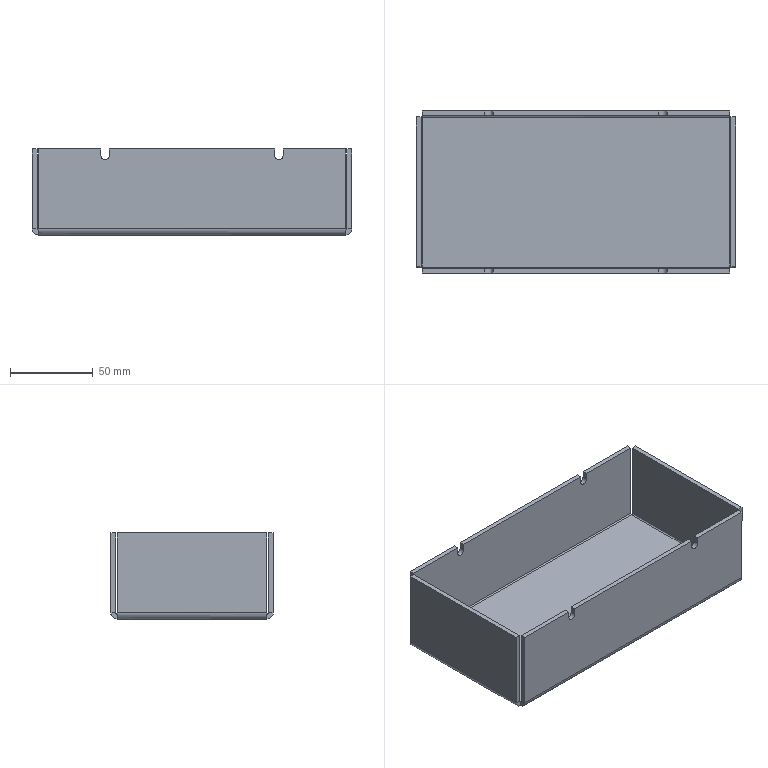Part | SolidWorks | features EdgeFlange 1, FlatPattern 1, ICE 1, SMBaseFlange 1, SheetMetal 1 | 1 solid | 54 faces | box 193 x 98 x 52 mm | volume 135822 mm3 | plane 34 | cylinder 12 | spline 8 | commonest cylinder face diameters 1.473 x4 5 x4 7.473 x4